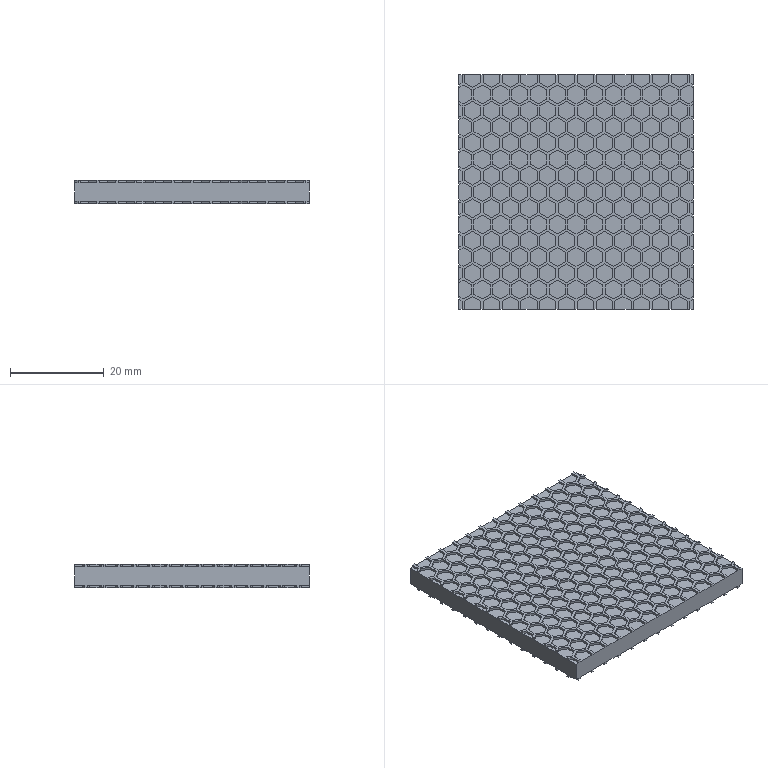Part | SolidWorks | features ICE 4, MirrorSolid 2, APattern 1, Extrusion 1 | 1 solid | 2620 faces | box 50 x 50 x 5 mm | volume 10617 mm3 | plane 2620